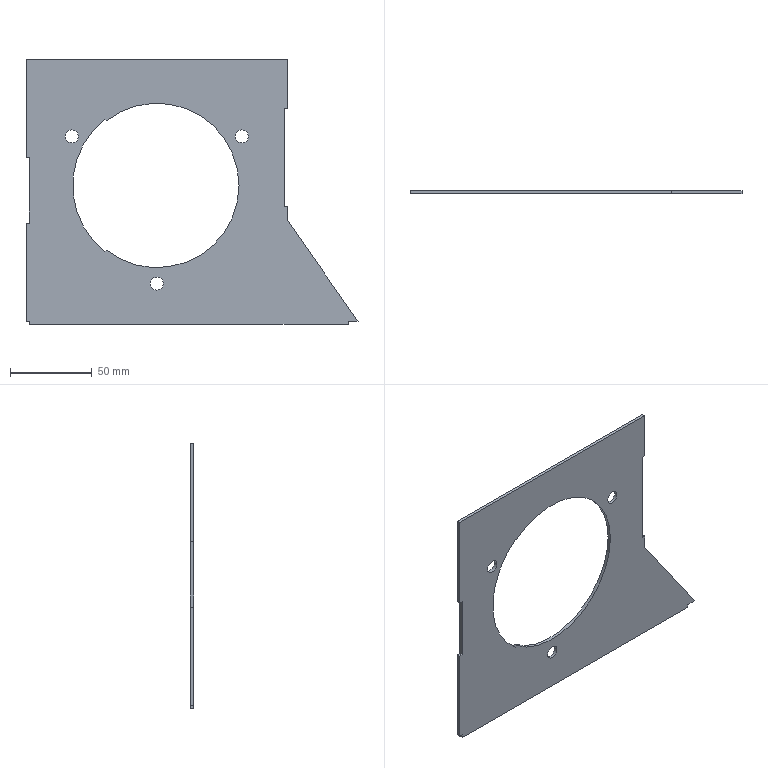Part | STEP file | JBJ-P-1003-02 | 1 solid | 26 faces | box 203 x 2 x 162 mm | volume 37833 mm3 | plane 21 | cylinder 5 | commonest cylinder face diameters 8 x3 100.5 x1 102.9 x1
STEP:
#1=CARTESIAN_POINT('',(80.,2.,-10.));
#2=VERTEX_POINT('',#1);
#3=CARTESIAN_POINT('',(80.,2.,-18.59));
#4=VERTEX_POINT('',#3);
#5=CARTESIAN_POINT('',(80.,2.,-18.59));
#6=DIRECTION('',(0.,0.,-1.));
#7=VECTOR('',#6,1000.);
#8=LINE('',#5,#7);
#9=EDGE_CURVE('',#2,#4,#8,.T.);
#10=ORIENTED_EDGE('',*,*,#9,.F.);
#11=CARTESIAN_POINT('',(80.,0.,-10.));
#12=VERTEX_POINT('',#11);
#13=CARTESIAN_POINT('',(80.,0.,-10.));
#14=DIRECTION('',(0.,1.,0.));
#15=VECTOR('',#14,1000.);
#16=LINE('',#13,#15);
#17=EDGE_CURVE('',#12,#2,#16,.T.);
#18=ORIENTED_EDGE('',*,*,#17,.F.);
#19=CARTESIAN_POINT('',(80.,0.,-18.59));
#20=VERTEX_POINT('',#19);
#21=CARTESIAN_POINT('',(80.,0.,-18.59));
#22=DIRECTION('',(0.,0.,-1.));
#23=VECTOR('',#22,1000.);
#24=LINE('',#21,#23);
#25=EDGE_CURVE('',#12,#20,#24,.T.);
#26=ORIENTED_EDGE('',*,*,#25,.T.);
#27=CARTESIAN_POINT('',(80.,2.,-18.59));
#28=DIRECTION('',(0.,-1.,0.));
#29=VECTOR('',#28,1000.);
#30=LINE('',#27,#29);
#31=EDGE_CURVE('',#4,#20,#30,.T.);
#32=ORIENTED_EDGE('',*,*,#31,.F.);
#33=EDGE_LOOP('',(#10,#18,#26,#32));
#34=FACE_OUTER_BOUND('',#33,.T.);
#35=CARTESIAN_POINT('',(80.,2.,-18.59));
#36=DIRECTION('',(-1.,0.,0.));
#37=DIRECTION('',(0.,0.,1.));
#38=AXIS2_PLACEMENT_3D('',#35,#36,#37);
#39=PLANE('',#38);
#40=ADVANCED_FACE('',(#34),#39,.F.);
#41=CARTESIAN_POINT('',(-80.,0.,-80.));
#42=VERTEX_POINT('',#41);
#43=CARTESIAN_POINT('',(-80.,0.,-20.));
#44=VERTEX_POINT('',#43);
#45=CARTESIAN_POINT('',(-80.,0.,-80.));
#46=DIRECTION('',(0.,0.,1.));
#47=VECTOR('',#46,1000.);
#48=LINE('',#45,#47);
#49=EDGE_CURVE('',#42,#44,#48,.T.);
#50=ORIENTED_EDGE('',*,*,#49,.T.);
#51=CARTESIAN_POINT('',(-80.,2.,-20.));
#52=VERTEX_POINT('',#51);
#53=CARTESIAN_POINT('',(-80.,2.,-20.));
#54=DIRECTION('',(0.,-1.,0.));
#55=VECTOR('',#54,1000.);
#56=LINE('',#53,#55);
#57=EDGE_CURVE('',#52,#44,#56,.T.);
#58=ORIENTED_EDGE('',*,*,#57,.F.);
#59=CARTESIAN_POINT('',(-80.,2.,-80.));
#60=VERTEX_POINT('',#59);
#61=CARTESIAN_POINT('',(-80.,2.,-80.));
#62=DIRECTION('',(0.,0.,1.));
#63=VECTOR('',#62,1000.);
#64=LINE('',#61,#63);
#65=EDGE_CURVE('',#60,#52,#64,.T.);
#66=ORIENTED_EDGE('',*,*,#65,.F.);
#67=CARTESIAN_POINT('',(-80.,2.,-80.));
#68=DIRECTION('',(0.,-1.,0.));
#69=VECTOR('',#68,1000.);
#70=LINE('',#67,#69);
#71=EDGE_CURVE('',#60,#42,#70,.T.);
#72=ORIENTED_EDGE('',*,*,#71,.T.);
#73=EDGE_LOOP('',(#50,#58,#66,#72));
#74=FACE_OUTER_BOUND('',#73,.T.);
#75=CARTESIAN_POINT('',(-80.,2.,-80.));
#76=DIRECTION('',(1.,0.,0.));
#77=DIRECTION('',(0.,0.,-1.));
#78=AXIS2_PLACEMENT_3D('',#75,#76,#77);
#79=PLANE('',#78);
#80=ADVANCED_FACE('',(#74),#79,.F.);
#81=CARTESIAN_POINT('',(-78.,0.,-80.));
#82=VERTEX_POINT('',#81);
#83=CARTESIAN_POINT('',(-78.,2.,-80.));
#84=VERTEX_POINT('',#83);
#85=CARTESIAN_POINT('',(-78.,0.,-80.));
#86=DIRECTION('',(0.,1.,0.));
#87=VECTOR('',#86,1000.);
#88=LINE('',#85,#87);
#89=EDGE_CURVE('',#82,#84,#88,.T.);
#90=ORIENTED_EDGE('',*,*,#89,.F.);
#91=CARTESIAN_POINT('',(-80.,0.,-80.));
#92=DIRECTION('',(-1.,0.,0.));
#93=VECTOR('',#92,1000.);
#94=LINE('',#91,#93);
#95=EDGE_CURVE('',#82,#42,#94,.T.);
#96=ORIENTED_EDGE('',*,*,#95,.T.);
#97=ORIENTED_EDGE('',*,*,#71,.F.);
#98=CARTESIAN_POINT('',(-80.,2.,-80.));
#99=DIRECTION('',(-1.,0.,0.));
#100=VECTOR('',#99,1000.);
#101=LINE('',#98,#100);
#102=EDGE_CURVE('',#84,#60,#101,.T.);
#103=ORIENTED_EDGE('',*,*,#102,.F.);
#104=EDGE_LOOP('',(#90,#96,#97,#103));
#105=FACE_OUTER_BOUND('',#104,.T.);
#106=CARTESIAN_POINT('',(-80.,2.,-80.));
#107=DIRECTION('',(0.,0.,1.));
#108=DIRECTION('',(1.,0.,0.));
#109=AXIS2_PLACEMENT_3D('',#106,#107,#108);
#110=PLANE('',#109);
#111=ADVANCED_FACE('',(#105),#110,.F.);
#112=CARTESIAN_POINT('',(117.,2.,-80.));
#113=VERTEX_POINT('',#112);
#114=CARTESIAN_POINT('',(117.,0.,-80.));
#115=VERTEX_POINT('',#114);
#116=CARTESIAN_POINT('',(117.,2.,-80.));
#117=DIRECTION('',(0.,-1.,0.));
#118=VECTOR('',#117,1000.);
#119=LINE('',#116,#118);
#120=EDGE_CURVE('',#113,#115,#119,.T.);
#121=ORIENTED_EDGE('',*,*,#120,.F.);
#122=CARTESIAN_POINT('',(123.,2.,-80.));
#123=VERTEX_POINT('',#122);
#124=CARTESIAN_POINT('',(-80.,2.,-80.));
#125=DIRECTION('',(-1.,0.,0.));
#126=VECTOR('',#125,1000.);
#127=LINE('',#124,#126);
#128=EDGE_CURVE('',#123,#113,#127,.T.);
#129=ORIENTED_EDGE('',*,*,#128,.F.);
#130=CARTESIAN_POINT('',(123.,0.,-80.));
#131=VERTEX_POINT('',#130);
#132=CARTESIAN_POINT('',(123.,2.,-80.));
#133=DIRECTION('',(0.,-1.,0.));
#134=VECTOR('',#133,1000.);
#135=LINE('',#132,#134);
#136=EDGE_CURVE('',#123,#131,#135,.T.);
#137=ORIENTED_EDGE('',*,*,#136,.T.);
#138=CARTESIAN_POINT('',(-80.,0.,-80.));
#139=DIRECTION('',(-1.,0.,0.));
#140=VECTOR('',#139,1000.);
#141=LINE('',#138,#140);
#142=EDGE_CURVE('',#131,#115,#141,.T.);
#143=ORIENTED_EDGE('',*,*,#142,.T.);
#144=EDGE_LOOP('',(#121,#129,#137,#143));
#145=FACE_OUTER_BOUND('',#144,.T.);
#146=CARTESIAN_POINT('',(-80.,2.,-80.));
#147=DIRECTION('',(0.,0.,1.));
#148=DIRECTION('',(1.,0.,0.));
#149=AXIS2_PLACEMENT_3D('',#146,#147,#148);
#150=PLANE('',#149);
#151=ADVANCED_FACE('',(#145),#150,.F.);
#152=CARTESIAN_POINT('',(80.,0.,80.));
#153=VERTEX_POINT('',#152);
#154=CARTESIAN_POINT('',(80.,0.,50.));
#155=VERTEX_POINT('',#154);
#156=CARTESIAN_POINT('',(80.,0.,-18.59));
#157=DIRECTION('',(0.,0.,-1.));
#158=VECTOR('',#157,1000.);
#159=LINE('',#156,#158);
#160=EDGE_CURVE('',#153,#155,#159,.T.);
#161=ORIENTED_EDGE('',*,*,#160,.T.);
#162=CARTESIAN_POINT('',(80.,2.,50.));
#163=VERTEX_POINT('',#162);
#164=CARTESIAN_POINT('',(80.,0.,50.));
#165=DIRECTION('',(0.,1.,0.));
#166=VECTOR('',#165,1000.);
#167=LINE('',#164,#166);
#168=EDGE_CURVE('',#155,#163,#167,.T.);
#169=ORIENTED_EDGE('',*,*,#168,.T.);
#170=CARTESIAN_POINT('',(80.,2.,80.));
#171=VERTEX_POINT('',#170);
#172=CARTESIAN_POINT('',(80.,2.,-18.59));
#173=DIRECTION('',(0.,0.,-1.));
#174=VECTOR('',#173,1000.);
#175=LINE('',#172,#174);
#176=EDGE_CURVE('',#171,#163,#175,.T.);
#177=ORIENTED_EDGE('',*,*,#176,.F.);
#178=CARTESIAN_POINT('',(80.,2.,80.));
#179=DIRECTION('',(0.,-1.,0.));
#180=VECTOR('',#179,1000.);
#181=LINE('',#178,#180);
#182=EDGE_CURVE('',#171,#153,#181,.T.);
#183=ORIENTED_EDGE('',*,*,#182,.T.);
#184=EDGE_LOOP('',(#161,#169,#177,#183));
#185=FACE_OUTER_BOUND('',#184,.T.);
#186=CARTESIAN_POINT('',(80.,2.,-18.59));
#187=DIRECTION('',(-1.,0.,0.));
#188=DIRECTION('',(0.,0.,1.));
#189=AXIS2_PLACEMENT_3D('',#186,#187,#188);
#190=PLANE('',#189);
#191=ADVANCED_FACE('',(#185),#190,.F.);
#192=CARTESIAN_POINT('',(123.,0.,-80.));
#193=DIRECTION('',(0.5736,0.,-0.8192));
#194=VECTOR('',#193,1000.);
#195=LINE('',#192,#194);
#196=EDGE_CURVE('',#20,#131,#195,.T.);
#197=ORIENTED_EDGE('',*,*,#196,.T.);
#198=ORIENTED_EDGE('',*,*,#136,.F.);
#199=CARTESIAN_POINT('',(123.,2.,-80.));
#200=DIRECTION('',(0.5736,0.,-0.8192));
#201=VECTOR('',#200,1000.);
#202=LINE('',#199,#201);
#203=EDGE_CURVE('',#4,#123,#202,.T.);
#204=ORIENTED_EDGE('',*,*,#203,.F.);
#205=ORIENTED_EDGE('',*,*,#31,.T.);
#206=EDGE_LOOP('',(#197,#198,#204,#205));
#207=FACE_OUTER_BOUND('',#206,.T.);
#208=CARTESIAN_POINT('',(123.,2.,-80.));
#209=DIRECTION('',(-0.8192,0.,-0.5736));
#210=DIRECTION('',(-0.5736,0.,0.8192));
#211=AXIS2_PLACEMENT_3D('',#208,#209,#210);
#212=PLANE('',#211);
#213=ADVANCED_FACE('',(#207),#212,.F.);
#214=CARTESIAN_POINT('',(-80.,2.,20.));
#215=VERTEX_POINT('',#214);
#216=CARTESIAN_POINT('',(-80.,2.,80.));
#217=VERTEX_POINT('',#216);
#218=CARTESIAN_POINT('',(-80.,2.,-80.));
#219=DIRECTION('',(0.,0.,1.));
#220=VECTOR('',#219,1000.);
#221=LINE('',#218,#220);
#222=EDGE_CURVE('',#215,#217,#221,.T.);
#223=ORIENTED_EDGE('',*,*,#222,.F.);
#224=CARTESIAN_POINT('',(-80.,0.,20.));
#225=VERTEX_POINT('',#224);
#226=CARTESIAN_POINT('',(-80.,2.,20.));
#227=DIRECTION('',(0.,-1.,0.));
#228=VECTOR('',#227,1000.);
#229=LINE('',#226,#228);
#230=EDGE_CURVE('',#215,#225,#229,.T.);
#231=ORIENTED_EDGE('',*,*,#230,.T.);
#232=CARTESIAN_POINT('',(-80.,0.,80.));
#233=VERTEX_POINT('',#232);
#234=CARTESIAN_POINT('',(-80.,0.,-80.));
#235=DIRECTION('',(0.,0.,1.));
#236=VECTOR('',#235,1000.);
#237=LINE('',#234,#236);
#238=EDGE_CURVE('',#225,#233,#237,.T.);
#239=ORIENTED_EDGE('',*,*,#238,.T.);
#240=CARTESIAN_POINT('',(-80.,2.,80.));
#241=DIRECTION('',(0.,-1.,0.));
#242=VECTOR('',#241,1000.);
#243=LINE('',#240,#242);
#244=EDGE_CURVE('',#217,#233,#243,.T.);
#245=ORIENTED_EDGE('',*,*,#244,.F.);
#246=EDGE_LOOP('',(#223,#231,#239,#245));
#247=FACE_OUTER_BOUND('',#246,.T.);
#248=CARTESIAN_POINT('',(-80.,2.,-80.));
#249=DIRECTION('',(1.,0.,0.));
#250=DIRECTION('',(0.,0.,-1.));
#251=AXIS2_PLACEMENT_3D('',#248,#249,#250);
#252=PLANE('',#251);
#253=ADVANCED_FACE('',(#247),#252,.F.);
#254=CARTESIAN_POINT('',(-80.,0.,80.));
#255=DIRECTION('',(1.,0.,0.));
#256=VECTOR('',#255,1000.);
#257=LINE('',#254,#256);
#258=EDGE_CURVE('',#233,#153,#257,.T.);
#259=ORIENTED_EDGE('',*,*,#258,.T.);
#260=ORIENTED_EDGE('',*,*,#182,.F.);
#261=CARTESIAN_POINT('',(-80.,2.,80.));
#262=DIRECTION('',(1.,0.,0.));
#263=VECTOR('',#262,1000.);
#264=LINE('',#261,#263);
#265=EDGE_CURVE('',#217,#171,#264,.T.);
#266=ORIENTED_EDGE('',*,*,#265,.F.);
#267=ORIENTED_EDGE('',*,*,#244,.T.);
#268=EDGE_LOOP('',(#259,#260,#266,#267));
#269=FACE_OUTER_BOUND('',#268,.T.);
#270=CARTESIAN_POINT('',(-80.,2.,80.));
#271=DIRECTION('',(0.,0.,-1.));
#272=DIRECTION('',(-1.,0.,0.));
#273=AXIS2_PLACEMENT_3D('',#270,#271,#272);
#274=PLANE('',#273);
#275=ADVANCED_FACE('',(#269),#274,.F.);
#276=CARTESIAN_POINT('',(-31.061,2.,-36.5));
#277=VERTEX_POINT('',#276);
#278=CARTESIAN_POINT('',(-31.803,2.,-37.443));
#279=VERTEX_POINT('',#278);
#280=CARTESIAN_POINT('',(-31.803,2.,-37.443));
#281=DIRECTION('',(-0.6181,0.,-0.7861));
#282=VECTOR('',#281,1000.);
#283=LINE('',#280,#282);
#284=EDGE_CURVE('',#277,#279,#283,.T.);
#285=ORIENTED_EDGE('',*,*,#284,.F.);
#286=CARTESIAN_POINT('',(-31.061,2.,42.5));
#287=VERTEX_POINT('',#286);
#288=CARTESIAN_POINT('',(0.,2.,3.));
#289=DIRECTION('',(0.,1.,0.));
#290=DIRECTION('',(0.,0.,1.));
#291=AXIS2_PLACEMENT_3D('',#288,#289,#290);
#292=CIRCLE('',#291,50.25);
#293=EDGE_CURVE('',#287,#277,#292,.T.);
#294=ORIENTED_EDGE('',*,*,#293,.F.);
#295=CARTESIAN_POINT('',(-31.803,2.,43.443));
#296=VERTEX_POINT('',#295);
#297=CARTESIAN_POINT('',(-31.803,2.,43.443));
#298=DIRECTION('',(0.6181,0.,-0.7861));
#299=VECTOR('',#298,1000.);
#300=LINE('',#297,#299);
#301=EDGE_CURVE('',#296,#287,#300,.T.);
#302=ORIENTED_EDGE('',*,*,#301,.F.);
#303=CARTESIAN_POINT('',(0.,2.,3.));
#304=DIRECTION('',(0.,1.,0.));
#305=DIRECTION('',(0.,0.,1.));
#306=AXIS2_PLACEMENT_3D('',#303,#304,#305);
#307=CIRCLE('',#306,51.45);
#308=EDGE_CURVE('',#279,#296,#307,.T.);
#309=ORIENTED_EDGE('',*,*,#308,.F.);
#310=EDGE_LOOP('',(#285,#294,#302,#309));
#311=FACE_BOUND('',#310,.T.);
#312=CARTESIAN_POINT('',(0.,2.,-61.));
#313=VERTEX_POINT('',#312);
#314=CARTESIAN_POINT('',(0.,2.,-57.));
#315=DIRECTION('',(0.,-1.,0.));
#316=DIRECTION('',(0.,0.,-1.));
#317=AXIS2_PLACEMENT_3D('',#314,#315,#316);
#318=CIRCLE('',#317,4.);
#319=EDGE_CURVE('',#313,#313,#318,.T.);
#320=ORIENTED_EDGE('',*,*,#319,.T.);
#321=EDGE_LOOP('',(#320));
#322=FACE_BOUND('',#321,.T.);
#323=CARTESIAN_POINT('',(-51.962,2.,29.));
#324=VERTEX_POINT('',#323);
#325=CARTESIAN_POINT('',(-51.962,2.,33.));
#326=DIRECTION('',(0.,-1.,0.));
#327=DIRECTION('',(0.,0.,-1.));
#328=AXIS2_PLACEMENT_3D('',#325,#326,#327);
#329=CIRCLE('',#328,4.);
#330=EDGE_CURVE('',#324,#324,#329,.T.);
#331=ORIENTED_EDGE('',*,*,#330,.T.);
#332=EDGE_LOOP('',(#331));
#333=FACE_BOUND('',#332,.T.);
#334=CARTESIAN_POINT('',(51.962,2.,29.));
#335=VERTEX_POINT('',#334);
#336=CARTESIAN_POINT('',(51.962,2.,33.));
#337=DIRECTION('',(0.,-1.,0.));
#338=DIRECTION('',(0.,0.,-1.));
#339=AXIS2_PLACEMENT_3D('',#336,#337,#338);
#340=CIRCLE('',#339,4.);
#341=EDGE_CURVE('',#335,#335,#340,.T.);
#342=ORIENTED_EDGE('',*,*,#341,.T.);
#343=EDGE_LOOP('',(#342));
#344=FACE_BOUND('',#343,.T.);
#345=CARTESIAN_POINT('',(78.,2.,-10.));
#346=VERTEX_POINT('',#345);
#347=CARTESIAN_POINT('',(78.,2.,-10.));
#348=DIRECTION('',(-1.,0.,0.));
#349=VECTOR('',#348,1000.);
#350=LINE('',#347,#349);
#351=EDGE_CURVE('',#2,#346,#350,.T.);
#352=ORIENTED_EDGE('',*,*,#351,.F.);
#353=ORIENTED_EDGE('',*,*,#9,.T.);
#354=ORIENTED_EDGE('',*,*,#203,.T.);
#355=ORIENTED_EDGE('',*,*,#128,.T.);
#356=CARTESIAN_POINT('',(117.,2.,-82.));
#357=VERTEX_POINT('',#356);
#358=CARTESIAN_POINT('',(117.,2.,-82.));
#359=DIRECTION('',(0.,0.,1.));
#360=VECTOR('',#359,1000.);
#361=LINE('',#358,#360);
#362=EDGE_CURVE('',#357,#113,#361,.T.);
#363=ORIENTED_EDGE('',*,*,#362,.F.);
#364=CARTESIAN_POINT('',(-78.,2.,-82.));
#365=VERTEX_POINT('',#364);
#366=CARTESIAN_POINT('',(-78.,2.,-82.));
#367=DIRECTION('',(1.,0.,0.));
#368=VECTOR('',#367,1000.);
#369=LINE('',#366,#368);
#370=EDGE_CURVE('',#365,#357,#369,.T.);
#371=ORIENTED_EDGE('',*,*,#370,.F.);
#372=CARTESIAN_POINT('',(-78.,2.,-82.));
#373=DIRECTION('',(0.,0.,1.));
#374=VECTOR('',#373,1000.);
#375=LINE('',#372,#374);
#376=EDGE_CURVE('',#365,#84,#375,.T.);
#377=ORIENTED_EDGE('',*,*,#376,.T.);
#378=ORIENTED_EDGE('',*,*,#102,.T.);
#379=ORIENTED_EDGE('',*,*,#65,.T.);
#380=CARTESIAN_POINT('',(-78.,2.,-20.));
#381=VERTEX_POINT('',#380);
#382=CARTESIAN_POINT('',(-78.,2.,-20.));
#383=DIRECTION('',(1.,0.,0.));
#384=VECTOR('',#383,1000.);
#385=LINE('',#382,#384);
#386=EDGE_CURVE('',#52,#381,#385,.T.);
#387=ORIENTED_EDGE('',*,*,#386,.T.);
#388=CARTESIAN_POINT('',(-78.,2.,20.));
#389=VERTEX_POINT('',#388);
#390=CARTESIAN_POINT('',(-78.,2.,-20.));
#391=DIRECTION('',(0.,0.,1.));
#392=VECTOR('',#391,1000.);
#393=LINE('',#390,#392);
#394=EDGE_CURVE('',#381,#389,#393,.T.);
#395=ORIENTED_EDGE('',*,*,#394,.T.);
#396=CARTESIAN_POINT('',(-78.,2.,20.));
#397=DIRECTION('',(-1.,0.,0.));
#398=VECTOR('',#397,1000.);
#399=LINE('',#396,#398);
#400=EDGE_CURVE('',#389,#215,#399,.T.);
#401=ORIENTED_EDGE('',*,*,#400,.T.);
#402=ORIENTED_EDGE('',*,*,#222,.T.);
#403=ORIENTED_EDGE('',*,*,#265,.T.);
#404=ORIENTED_EDGE('',*,*,#176,.T.);
#405=CARTESIAN_POINT('',(78.,2.,50.));
#406=VERTEX_POINT('',#405);
#407=CARTESIAN_POINT('',(78.,2.,50.));
#408=DIRECTION('',(1.,0.,0.));
#409=VECTOR('',#408,1000.);
#410=LINE('',#407,#409);
#411=EDGE_CURVE('',#406,#163,#410,.T.);
#412=ORIENTED_EDGE('',*,*,#411,.F.);
#413=CARTESIAN_POINT('',(78.,2.,-10.));
#414=DIRECTION('',(0.,0.,1.));
#415=VECTOR('',#414,1000.);
#416=LINE('',#413,#415);
#417=EDGE_CURVE('',#346,#406,#416,.T.);
#418=ORIENTED_EDGE('',*,*,#417,.F.);
#419=EDGE_LOOP('',(#352,#353,#354,#355,#363,#371,#377,#378,#379,#387,#395,#401,#402,#403,#404,#412,#418));
#420=FACE_OUTER_BOUND('',#419,.T.);
#421=CARTESIAN_POINT('',(0.,2.,0.));
#422=DIRECTION('',(0.,1.,0.));
#423=DIRECTION('',(0.,0.,1.));
#424=AXIS2_PLACEMENT_3D('',#421,#422,#423);
#425=PLANE('',#424);
#426=ADVANCED_FACE('',(#311,#322,#333,#344,#420),#425,.T.);
#427=CARTESIAN_POINT('',(0.,0.,-61.));
#428=VERTEX_POINT('',#427);
#429=CARTESIAN_POINT('',(0.,0.,-57.));
#430=DIRECTION('',(0.,-1.,0.));
#431=DIRECTION('',(0.,0.,-1.));
#432=AXIS2_PLACEMENT_3D('',#429,#430,#431);
#433=CIRCLE('',#432,4.);
#434=EDGE_CURVE('',#428,#428,#433,.T.);
#435=ORIENTED_EDGE('',*,*,#434,.F.);
#436=EDGE_LOOP('',(#435));
#437=FACE_BOUND('',#436,.T.);
#438=CARTESIAN_POINT('',(-51.962,0.,29.));
#439=VERTEX_POINT('',#438);
#440=CARTESIAN_POINT('',(-51.962,0.,33.));
#441=DIRECTION('',(0.,-1.,0.));
#442=DIRECTION('',(0.,0.,-1.));
#443=AXIS2_PLACEMENT_3D('',#440,#441,#442);
#444=CIRCLE('',#443,4.);
#445=EDGE_CURVE('',#439,#439,#444,.T.);
#446=ORIENTED_EDGE('',*,*,#445,.F.);
#447=EDGE_LOOP('',(#446));
#448=FACE_BOUND('',#447,.T.);
#449=CARTESIAN_POINT('',(51.962,0.,29.));
#450=VERTEX_POINT('',#449);
#451=CARTESIAN_POINT('',(51.962,0.,33.));
#452=DIRECTION('',(0.,-1.,0.));
#453=DIRECTION('',(0.,0.,-1.));
#454=AXIS2_PLACEMENT_3D('',#451,#452,#453);
#455=CIRCLE('',#454,4.);
#456=EDGE_CURVE('',#450,#450,#455,.T.);
#457=ORIENTED_EDGE('',*,*,#456,.F.);
#458=EDGE_LOOP('',(#457));
#459=FACE_BOUND('',#458,.T.);
#460=CARTESIAN_POINT('',(-31.061,0.,-36.5));
#461=VERTEX_POINT('',#460);
#462=CARTESIAN_POINT('',(-31.061,0.,42.5));
#463=VERTEX_POINT('',#462);
#464=CARTESIAN_POINT('',(0.,0.,3.));
#465=DIRECTION('',(0.,-1.,0.));
#466=DIRECTION('',(0.,0.,-1.));
#467=AXIS2_PLACEMENT_3D('',#464,#465,#466);
#468=CIRCLE('',#467,50.25);
#469=EDGE_CURVE('',#461,#463,#468,.T.);
#470=ORIENTED_EDGE('',*,*,#469,.F.);
#471=CARTESIAN_POINT('',(-31.803,0.,-37.443));
#472=VERTEX_POINT('',#471);
#473=CARTESIAN_POINT('',(-1.458,0.,1.146));
#474=DIRECTION('',(-0.6181,0.,-0.7861));
#475=VECTOR('',#474,1000.);
#476=LINE('',#473,#475);
#477=EDGE_CURVE('',#461,#472,#476,.T.);
#478=ORIENTED_EDGE('',*,*,#477,.T.);
#479=CARTESIAN_POINT('',(-31.803,0.,43.443));
#480=VERTEX_POINT('',#479);
#481=CARTESIAN_POINT('',(0.,0.,3.));
#482=DIRECTION('',(0.,1.,0.));
#483=DIRECTION('',(0.,0.,1.));
#484=AXIS2_PLACEMENT_3D('',#481,#482,#483);
#485=CIRCLE('',#484,51.45);
#486=EDGE_CURVE('',#472,#480,#485,.T.);
#487=ORIENTED_EDGE('',*,*,#486,.T.);
#488=CARTESIAN_POINT('',(1.458,0.,1.146));
#489=DIRECTION('',(0.6181,0.,-0.7861));
#490=VECTOR('',#489,1000.);
#491=LINE('',#488,#490);
#492=EDGE_CURVE('',#480,#463,#491,.T.);
#493=ORIENTED_EDGE('',*,*,#492,.T.);
#494=EDGE_LOOP('',(#470,#478,#487,#493));
#495=FACE_BOUND('',#494,.T.);
#496=ORIENTED_EDGE('',*,*,#25,.F.);
#497=CARTESIAN_POINT('',(78.,0.,-10.));
#498=VERTEX_POINT('',#497);
#499=CARTESIAN_POINT('',(78.,0.,-10.));
#500=DIRECTION('',(-1.,0.,0.));
#501=VECTOR('',#500,1000.);
#502=LINE('',#499,#501);
#503=EDGE_CURVE('',#12,#498,#502,.T.);
#504=ORIENTED_EDGE('',*,*,#503,.T.);
#505=CARTESIAN_POINT('',(78.,0.,50.));
#506=VERTEX_POINT('',#505);
#507=CARTESIAN_POINT('',(78.,0.,-10.));
#508=DIRECTION('',(0.,0.,1.));
#509=VECTOR('',#508,1000.);
#510=LINE('',#507,#509);
#511=EDGE_CURVE('',#498,#506,#510,.T.);
#512=ORIENTED_EDGE('',*,*,#511,.T.);
#513=CARTESIAN_POINT('',(78.,0.,50.));
#514=DIRECTION('',(1.,0.,0.));
#515=VECTOR('',#514,1000.);
#516=LINE('',#513,#515);
#517=EDGE_CURVE('',#506,#155,#516,.T.);
#518=ORIENTED_EDGE('',*,*,#517,.T.);
#519=ORIENTED_EDGE('',*,*,#160,.F.);
#520=ORIENTED_EDGE('',*,*,#258,.F.);
#521=ORIENTED_EDGE('',*,*,#238,.F.);
#522=CARTESIAN_POINT('',(-78.,0.,20.));
#523=VERTEX_POINT('',#522);
#524=CARTESIAN_POINT('',(-78.,0.,20.));
#525=DIRECTION('',(-1.,0.,0.));
#526=VECTOR('',#525,1000.);
#527=LINE('',#524,#526);
#528=EDGE_CURVE('',#523,#225,#527,.T.);
#529=ORIENTED_EDGE('',*,*,#528,.F.);
#530=CARTESIAN_POINT('',(-78.,0.,-20.));
#531=VERTEX_POINT('',#530);
#532=CARTESIAN_POINT('',(-78.,0.,-20.));
#533=DIRECTION('',(0.,0.,1.));
#534=VECTOR('',#533,1000.);
#535=LINE('',#532,#534);
#536=EDGE_CURVE('',#531,#523,#535,.T.);
#537=ORIENTED_EDGE('',*,*,#536,.F.);
#538=CARTESIAN_POINT('',(-78.,0.,-20.));
#539=DIRECTION('',(1.,0.,0.));
#540=VECTOR('',#539,1000.);
#541=LINE('',#538,#540);
#542=EDGE_CURVE('',#44,#531,#541,.T.);
#543=ORIENTED_EDGE('',*,*,#542,.F.);
#544=ORIENTED_EDGE('',*,*,#49,.F.);
#545=ORIENTED_EDGE('',*,*,#95,.F.);
#546=CARTESIAN_POINT('',(-78.,0.,-82.));
#547=VERTEX_POINT('',#546);
#548=CARTESIAN_POINT('',(-78.,0.,-82.));
#549=DIRECTION('',(0.,0.,1.));
#550=VECTOR('',#549,1000.);
#551=LINE('',#548,#550);
#552=EDGE_CURVE('',#547,#82,#551,.T.);
#553=ORIENTED_EDGE('',*,*,#552,.F.);
#554=CARTESIAN_POINT('',(117.,0.,-82.));
#555=VERTEX_POINT('',#554);
#556=CARTESIAN_POINT('',(117.,0.,-82.));
#557=DIRECTION('',(-1.,0.,0.));
#558=VECTOR('',#557,1000.);
#559=LINE('',#556,#558);
#560=EDGE_CURVE('',#555,#547,#559,.T.);
#561=ORIENTED_EDGE('',*,*,#560,.F.);
#562=CARTESIAN_POINT('',(117.,0.,-82.));
#563=DIRECTION('',(0.,0.,1.));
#564=VECTOR('',#563,1000.);
#565=LINE('',#562,#564);
#566=EDGE_CURVE('',#555,#115,#565,.T.);
#567=ORIENTED_EDGE('',*,*,#566,.T.);
#568=ORIENTED_EDGE('',*,*,#142,.F.);
#569=ORIENTED_EDGE('',*,*,#196,.F.);
#570=EDGE_LOOP('',(#496,#504,#512,#518,#519,#520,#521,#529,#537,#543,#544,#545,#553,#561,#567,#568,#569));
#571=FACE_OUTER_BOUND('',#570,.T.);
#572=CARTESIAN_POINT('',(0.,0.,0.));
#573=DIRECTION('',(0.,1.,0.));
#574=DIRECTION('',(0.,0.,1.));
#575=AXIS2_PLACEMENT_3D('',#572,#573,#574);
#576=PLANE('',#575);
#577=ADVANCED_FACE('',(#437,#448,#459,#495,#571),#576,.F.);
#578=ORIENTED_EDGE('',*,*,#120,.T.);
#579=ORIENTED_EDGE('',*,*,#566,.F.);
#580=CARTESIAN_POINT('',(117.,2.,-82.));
#581=DIRECTION('',(0.,-1.,0.));
#582=VECTOR('',#581,1000.);
#583=LINE('',#580,#582);
#584=EDGE_CURVE('',#357,#555,#583,.T.);
#585=ORIENTED_EDGE('',*,*,#584,.F.);
#586=ORIENTED_EDGE('',*,*,#362,.T.);
#587=EDGE_LOOP('',(#578,#579,#585,#586));
#588=FACE_OUTER_BOUND('',#587,.T.);
#589=CARTESIAN_POINT('',(117.,2.,-82.));
#590=DIRECTION('',(-1.,0.,0.));
#591=DIRECTION('',(0.,0.,1.));
#592=AXIS2_PLACEMENT_3D('',#589,#590,#591);
#593=PLANE('',#592);
#594=ADVANCED_FACE('',(#588),#593,.F.);
#595=ORIENTED_EDGE('',*,*,#89,.T.);
#596=ORIENTED_EDGE('',*,*,#376,.F.);
#597=CARTESIAN_POINT('',(-78.,0.,-82.));
#598=DIRECTION('',(0.,1.,0.));
#599=VECTOR('',#598,1000.);
#600=LINE('',#597,#599);
#601=EDGE_CURVE('',#547,#365,#600,.T.);
#602=ORIENTED_EDGE('',*,*,#601,.F.);
#603=ORIENTED_EDGE('',*,*,#552,.T.);
#604=EDGE_LOOP('',(#595,#596,#602,#603));
#605=FACE_OUTER_BOUND('',#604,.T.);
#606=CARTESIAN_POINT('',(-78.,0.,-82.));
#607=DIRECTION('',(1.,0.,0.));
#608=DIRECTION('',(0.,1.,0.));
#609=AXIS2_PLACEMENT_3D('',#606,#607,#608);
#610=PLANE('',#609);
#611=ADVANCED_FACE('',(#605),#610,.F.);
#612=ORIENTED_EDGE('',*,*,#370,.T.);
#613=ORIENTED_EDGE('',*,*,#584,.T.);
#614=ORIENTED_EDGE('',*,*,#560,.T.);
#615=ORIENTED_EDGE('',*,*,#601,.T.);
#616=EDGE_LOOP('',(#612,#613,#614,#615));
#617=FACE_OUTER_BOUND('',#616,.T.);
#618=CARTESIAN_POINT('',(0.,0.,-82.));
#619=DIRECTION('',(0.,0.,-1.));
#620=DIRECTION('',(-1.,0.,0.));
#621=AXIS2_PLACEMENT_3D('',#618,#619,#620);
#622=PLANE('',#621);
#623=ADVANCED_FACE('',(#617),#622,.T.);
#624=ORIENTED_EDGE('',*,*,#293,.T.);
#625=CARTESIAN_POINT('',(-31.061,10.,-36.5));
#626=DIRECTION('',(0.,-1.,0.));
#627=VECTOR('',#626,1000.);
#628=LINE('',#625,#627);
#629=EDGE_CURVE('',#277,#461,#628,.T.);
#630=ORIENTED_EDGE('',*,*,#629,.T.);
#631=ORIENTED_EDGE('',*,*,#469,.T.);
#632=CARTESIAN_POINT('',(-31.061,10.,42.5));
#633=DIRECTION('',(0.,1.,0.));
#634=VECTOR('',#633,1000.);
#635=LINE('',#632,#634);
#636=EDGE_CURVE('',#463,#287,#635,.T.);
#637=ORIENTED_EDGE('',*,*,#636,.T.);
#638=EDGE_LOOP('',(#624,#630,#631,#637));
#639=FACE_OUTER_BOUND('',#638,.T.);
#640=CARTESIAN_POINT('',(0.,10.,3.));
#641=DIRECTION('',(0.,-1.,0.));
#642=DIRECTION('',(0.,0.,-1.));
#643=AXIS2_PLACEMENT_3D('',#640,#641,#642);
#644=CYLINDRICAL_SURFACE('',#643,50.25);
#645=ADVANCED_FACE('',(#639),#644,.F.);
#646=ORIENTED_EDGE('',*,*,#536,.T.);
#647=CARTESIAN_POINT('',(-78.,2.,20.));
#648=DIRECTION('',(0.,-1.,0.));
#649=VECTOR('',#648,1000.);
#650=LINE('',#647,#649);
#651=EDGE_CURVE('',#389,#523,#650,.T.);
#652=ORIENTED_EDGE('',*,*,#651,.F.);
#653=ORIENTED_EDGE('',*,*,#394,.F.);
#654=CARTESIAN_POINT('',(-78.,2.,-20.));
#655=DIRECTION('',(0.,-1.,0.));
#656=VECTOR('',#655,1000.);
#657=LINE('',#654,#656);
#658=EDGE_CURVE('',#381,#531,#657,.T.);
#659=ORIENTED_EDGE('',*,*,#658,.T.);
#660=EDGE_LOOP('',(#646,#652,#653,#659));
#661=FACE_OUTER_BOUND('',#660,.T.);
#662=CARTESIAN_POINT('',(-78.,2.,-20.));
#663=DIRECTION('',(1.,0.,0.));
#664=DIRECTION('',(0.,0.,-1.));
#665=AXIS2_PLACEMENT_3D('',#662,#663,#664);
#666=PLANE('',#665);
#667=ADVANCED_FACE('',(#661),#666,.F.);
#668=ORIENTED_EDGE('',*,*,#542,.T.);
#669=ORIENTED_EDGE('',*,*,#658,.F.);
#670=ORIENTED_EDGE('',*,*,#386,.F.);
#671=ORIENTED_EDGE('',*,*,#57,.T.);
#672=EDGE_LOOP('',(#668,#669,#670,#671));
#673=FACE_OUTER_BOUND('',#672,.T.);
#674=CARTESIAN_POINT('',(-78.,2.,-20.));
#675=DIRECTION('',(0.,0.,-1.));
#676=DIRECTION('',(-1.,0.,0.));
#677=AXIS2_PLACEMENT_3D('',#674,#675,#676);
#678=PLANE('',#677);
#679=ADVANCED_FACE('',(#673),#678,.F.);
#680=ORIENTED_EDGE('',*,*,#528,.T.);
#681=ORIENTED_EDGE('',*,*,#230,.F.);
#682=ORIENTED_EDGE('',*,*,#400,.F.);
#683=ORIENTED_EDGE('',*,*,#651,.T.);
#684=EDGE_LOOP('',(#680,#681,#682,#683));
#685=FACE_OUTER_BOUND('',#684,.T.);
#686=CARTESIAN_POINT('',(-78.,2.,20.));
#687=DIRECTION('',(0.,0.,1.));
#688=DIRECTION('',(1.,0.,0.));
#689=AXIS2_PLACEMENT_3D('',#686,#687,#688);
#690=PLANE('',#689);
#691=ADVANCED_FACE('',(#685),#690,.F.);
#692=ORIENTED_EDGE('',*,*,#417,.T.);
#693=CARTESIAN_POINT('',(78.,0.,50.));
#694=DIRECTION('',(0.,1.,0.));
#695=VECTOR('',#694,1000.);
#696=LINE('',#693,#695);
#697=EDGE_CURVE('',#506,#406,#696,.T.);
#698=ORIENTED_EDGE('',*,*,#697,.F.);
#699=ORIENTED_EDGE('',*,*,#511,.F.);
#700=CARTESIAN_POINT('',(78.,0.,-10.));
#701=DIRECTION('',(0.,1.,0.));
#702=VECTOR('',#701,1000.);
#703=LINE('',#700,#702);
#704=EDGE_CURVE('',#498,#346,#703,.T.);
#705=ORIENTED_EDGE('',*,*,#704,.T.);
#706=EDGE_LOOP('',(#692,#698,#699,#705));
#707=FACE_OUTER_BOUND('',#706,.T.);
#708=CARTESIAN_POINT('',(78.,0.,-10.));
#709=DIRECTION('',(-1.,0.,0.));
#710=DIRECTION('',(0.,0.,1.));
#711=AXIS2_PLACEMENT_3D('',#708,#709,#710);
#712=PLANE('',#711);
#713=ADVANCED_FACE('',(#707),#712,.F.);
#714=ORIENTED_EDGE('',*,*,#351,.T.);
#715=ORIENTED_EDGE('',*,*,#704,.F.);
#716=ORIENTED_EDGE('',*,*,#503,.F.);
#717=ORIENTED_EDGE('',*,*,#17,.T.);
#718=EDGE_LOOP('',(#714,#715,#716,#717));
#719=FACE_OUTER_BOUND('',#718,.T.);
#720=CARTESIAN_POINT('',(78.,0.,-10.));
#721=DIRECTION('',(0.,0.,-1.));
#722=DIRECTION('',(-1.,0.,0.));
#723=AXIS2_PLACEMENT_3D('',#720,#721,#722);
#724=PLANE('',#723);
#725=ADVANCED_FACE('',(#719),#724,.F.);
#726=ORIENTED_EDGE('',*,*,#411,.T.);
#727=ORIENTED_EDGE('',*,*,#168,.F.);
#728=ORIENTED_EDGE('',*,*,#517,.F.);
#729=ORIENTED_EDGE('',*,*,#697,.T.);
#730=EDGE_LOOP('',(#726,#727,#728,#729));
#731=FACE_OUTER_BOUND('',#730,.T.);
#732=CARTESIAN_POINT('',(78.,0.,50.));
#733=DIRECTION('',(0.,0.,1.));
#734=DIRECTION('',(1.,0.,0.));
#735=AXIS2_PLACEMENT_3D('',#732,#733,#734);
#736=PLANE('',#735);
#737=ADVANCED_FACE('',(#731),#736,.F.);
#738=ORIENTED_EDGE('',*,*,#341,.F.);
#739=EDGE_LOOP('',(#738));
#740=FACE_OUTER_BOUND('',#739,.T.);
#741=ORIENTED_EDGE('',*,*,#456,.T.);
#742=EDGE_LOOP('',(#741));
#743=FACE_OUTER_BOUND('',#742,.T.);
#744=CARTESIAN_POINT('',(51.962,2.,33.));
#745=DIRECTION('',(0.,-1.,0.));
#746=DIRECTION('',(0.,0.,-1.));
#747=AXIS2_PLACEMENT_3D('',#744,#745,#746);
#748=CYLINDRICAL_SURFACE('',#747,4.);
#749=ADVANCED_FACE('',(#740,#743),#748,.F.);
#750=ORIENTED_EDGE('',*,*,#330,.F.);
#751=EDGE_LOOP('',(#750));
#752=FACE_OUTER_BOUND('',#751,.T.);
#753=ORIENTED_EDGE('',*,*,#445,.T.);
#754=EDGE_LOOP('',(#753));
#755=FACE_OUTER_BOUND('',#754,.T.);
#756=CARTESIAN_POINT('',(-51.962,2.,33.));
#757=DIRECTION('',(0.,-1.,0.));
#758=DIRECTION('',(0.,0.,-1.));
#759=AXIS2_PLACEMENT_3D('',#756,#757,#758);
#760=CYLINDRICAL_SURFACE('',#759,4.);
#761=ADVANCED_FACE('',(#752,#755),#760,.F.);
#762=ORIENTED_EDGE('',*,*,#319,.F.);
#763=EDGE_LOOP('',(#762));
#764=FACE_OUTER_BOUND('',#763,.T.);
#765=ORIENTED_EDGE('',*,*,#434,.T.);
#766=EDGE_LOOP('',(#765));
#767=FACE_OUTER_BOUND('',#766,.T.);
#768=CARTESIAN_POINT('',(0.,2.,-57.));
#769=DIRECTION('',(0.,-1.,0.));
#770=DIRECTION('',(0.,0.,-1.));
#771=AXIS2_PLACEMENT_3D('',#768,#769,#770);
#772=CYLINDRICAL_SURFACE('',#771,4.);
#773=ADVANCED_FACE('',(#764,#767),#772,.F.);
#774=CARTESIAN_POINT('',(-31.803,-8.,-37.443));
#775=DIRECTION('',(0.,1.,0.));
#776=VECTOR('',#775,1000.);
#777=LINE('',#774,#776);
#778=EDGE_CURVE('',#472,#279,#777,.T.);
#779=ORIENTED_EDGE('',*,*,#778,.T.);
#780=ORIENTED_EDGE('',*,*,#308,.T.);
#781=CARTESIAN_POINT('',(-31.803,-8.,43.443));
#782=DIRECTION('',(0.,1.,0.));
#783=VECTOR('',#782,1000.);
#784=LINE('',#781,#783);
#785=EDGE_CURVE('',#480,#296,#784,.T.);
#786=ORIENTED_EDGE('',*,*,#785,.F.);
#787=ORIENTED_EDGE('',*,*,#486,.F.);
#788=EDGE_LOOP('',(#779,#780,#786,#787));
#789=FACE_OUTER_BOUND('',#788,.T.);
#790=CARTESIAN_POINT('',(0.,-8.,3.));
#791=DIRECTION('',(0.,1.,0.));
#792=DIRECTION('',(0.,0.,1.));
#793=AXIS2_PLACEMENT_3D('',#790,#791,#792);
#794=CYLINDRICAL_SURFACE('',#793,51.45);
#795=ADVANCED_FACE('',(#789),#794,.F.);
#796=ORIENTED_EDGE('',*,*,#629,.F.);
#797=ORIENTED_EDGE('',*,*,#284,.T.);
#798=ORIENTED_EDGE('',*,*,#778,.F.);
#799=ORIENTED_EDGE('',*,*,#477,.F.);
#800=EDGE_LOOP('',(#796,#797,#798,#799));
#801=FACE_OUTER_BOUND('',#800,.T.);
#802=CARTESIAN_POINT('',(-31.803,-8.,-37.443));
#803=DIRECTION('',(0.7861,0.,-0.6181));
#804=DIRECTION('',(-0.6181,0.,-0.7861));
#805=AXIS2_PLACEMENT_3D('',#802,#803,#804);
#806=PLANE('',#805);
#807=ADVANCED_FACE('',(#801),#806,.F.);
#808=ORIENTED_EDGE('',*,*,#785,.T.);
#809=ORIENTED_EDGE('',*,*,#301,.T.);
#810=ORIENTED_EDGE('',*,*,#636,.F.);
#811=ORIENTED_EDGE('',*,*,#492,.F.);
#812=EDGE_LOOP('',(#808,#809,#810,#811));
#813=FACE_OUTER_BOUND('',#812,.T.);
#814=CARTESIAN_POINT('',(-31.803,-8.,43.443));
#815=DIRECTION('',(0.7861,0.,0.6181));
#816=DIRECTION('',(0.6181,0.,-0.7861));
#817=AXIS2_PLACEMENT_3D('',#814,#815,#816);
#818=PLANE('',#817);
#819=ADVANCED_FACE('',(#813),#818,.F.);
#820=CLOSED_SHELL('',(#40,#80,#111,#151,#191,#213,#253,#275,#426,#577,#594,#611,#623,#645,#667,#679,#691,#713,#725,#737,#749,#761,#773,#795,#807,#819));
#821=MANIFOLD_SOLID_BREP('',#820);
#822=CARTESIAN_POINT('',(0.,0.,0.));
#823=DIRECTION('',(0.,0.,1.));
#824=DIRECTION('',(1.,0.,0.));
#825=AXIS2_PLACEMENT_3D('',#822,#823,#824);
#826=(LENGTH_UNIT()NAMED_UNIT(*)SI_UNIT(.MILLI.,.METRE.));
#827=UNCERTAINTY_MEASURE_WITH_UNIT(LENGTH_MEASURE(0.00001),#826,'','');
#828=(NAMED_UNIT(*)PLANE_ANGLE_UNIT()SI_UNIT($,.RADIAN.));
#829=(NAMED_UNIT(*)SI_UNIT($,.STERADIAN.)SOLID_ANGLE_UNIT());
#830=(GEOMETRIC_REPRESENTATION_CONTEXT(3)GLOBAL_UNCERTAINTY_ASSIGNED_CONTEXT((#827))GLOBAL_UNIT_ASSIGNED_CONTEXT((#826,#828,#829))REPRESENTATION_CONTEXT('',''));
#831=ADVANCED_BREP_SHAPE_REPRESENTATION('',(#821,#825),#830);